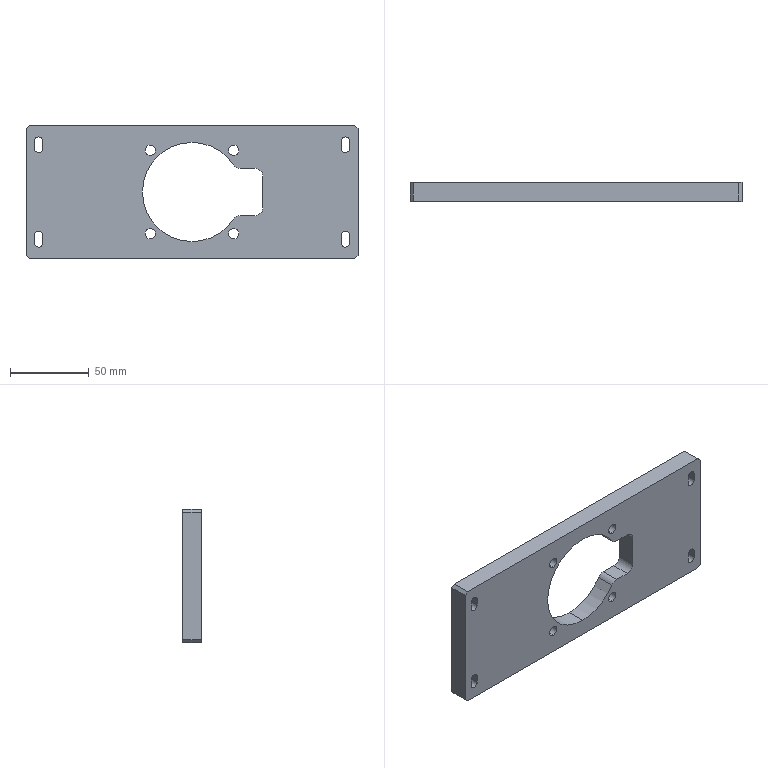Part | STEP file | 1105-104P042 | 1 solid | 84 faces | box 211 x 12 x 85 mm | volume 165704 mm3 | cylinder 47 | plane 37 | commonest cylinder face diameters 10 x16 5.5 x12 6.6 x8 11 x8 63 x3